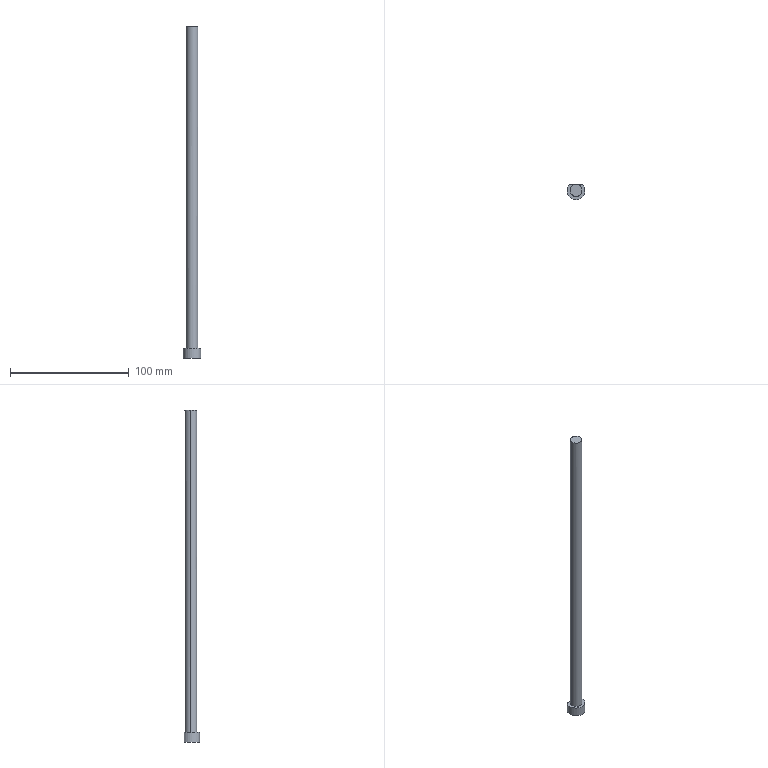Part | Creo | 1 solid | 7 faces | box 15 x 13 x 279.548 mm | volume 22625 mm3 | plane 4 | cylinder 3 | commonest cylinder face diameters 10 x2 15 x1
STEP:
#1=CARTESIAN_POINT('',(0.,0.,0.));
#2=DIRECTION('',(0.,0.,1.));
#3=DIRECTION('',(1.,0.,0.));
#4=AXIS2_PLACEMENT_3D('',#1,#2,#3);
#5=CARTESIAN_POINT('',(39.152,-157.9,-330.441));
#6=VERTEX_POINT('',#5);
#7=CARTESIAN_POINT('',(28.954,-157.9,-330.441));
#8=VERTEX_POINT('',#7);
#9=CARTESIAN_POINT('',(39.152,-157.9,-330.441));
#10=DIRECTION('',(-1.,0.,0.));
#11=VECTOR('',#10,10.198);
#12=LINE('',#9,#11);
#13=EDGE_CURVE('',#6,#8,#12,.T.);
#14=ORIENTED_EDGE('',*,*,#13,.F.);
#15=CARTESIAN_POINT('',(34.053,-163.4,-330.441));
#16=DIRECTION('',(0.,0.,-1.));
#17=DIRECTION('',(0.6799,0.7333,0.));
#18=AXIS2_PLACEMENT_3D('',#15,#16,#17);
#19=CIRCLE('',#18,7.5);
#20=EDGE_CURVE('',#6,#8,#19,.T.);
#21=ORIENTED_EDGE('',*,*,#20,.T.);
#22=EDGE_LOOP('',(#14,#21));
#23=FACE_OUTER_BOUND('',#22,.F.);
#24=CARTESIAN_POINT('',(29.053,-163.4,-330.441));
#25=VERTEX_POINT('',#24);
#26=CARTESIAN_POINT('',(39.053,-163.4,-330.441));
#27=VERTEX_POINT('',#26);
#28=CARTESIAN_POINT('',(34.053,-163.4,-330.441));
#29=DIRECTION('',(0.,0.,-1.));
#30=DIRECTION('',(-1.,0.,0.));
#31=AXIS2_PLACEMENT_3D('',#28,#29,#30);
#32=CIRCLE('',#31,5.);
#33=EDGE_CURVE('',#25,#27,#32,.T.);
#34=ORIENTED_EDGE('',*,*,#33,.F.);
#35=CARTESIAN_POINT('',(34.053,-163.4,-330.441));
#36=DIRECTION('',(0.,0.,-1.));
#37=DIRECTION('',(1.,0.,0.));
#38=AXIS2_PLACEMENT_3D('',#35,#36,#37);
#39=CIRCLE('',#38,5.);
#40=EDGE_CURVE('',#27,#25,#39,.T.);
#41=ORIENTED_EDGE('',*,*,#40,.F.);
#42=EDGE_LOOP('',(#34,#41));
#43=FACE_BOUND('',#42,.F.);
#44=CARTESIAN_POINT('',(34.053,-163.4,-330.441));
#45=DIRECTION('',(0.,0.,-1.));
#46=DIRECTION('',(-1.,0.,0.));
#47=AXIS2_PLACEMENT_3D('',#44,#45,#46);
#48=PLANE('',#47);
#49=ADVANCED_FACE('',(#23,#43),#48,.F.);
#50=CARTESIAN_POINT('',(39.053,-163.4,-58.958));
#51=VERTEX_POINT('',#50);
#52=CARTESIAN_POINT('',(34.383,-158.411,-58.894));
#53=VERTEX_POINT('',#52);
#54=CARTESIAN_POINT('',(39.053,-163.4,-58.958));
#55=CARTESIAN_POINT('',(39.053,-162.62,-58.947));
#56=CARTESIAN_POINT('',(38.729,-161.362,-58.93));
#57=CARTESIAN_POINT('',(37.774,-159.917,-58.911));
#58=CARTESIAN_POINT('',(36.394,-158.868,-58.898));
#59=CARTESIAN_POINT('',(35.161,-158.462,-58.894));
#60=B_SPLINE_CURVE_WITH_KNOTS('',3,(#54,#55,#56,#57,#58,#59,#52),.UNSPECIFIED.,.F.,.F.,(4,1,1,1,4),(0.,0.25,0.5,0.75,1.),.UNSPECIFIED.);
#61=EDGE_CURVE('',#51,#53,#60,.T.);
#62=ORIENTED_EDGE('',*,*,#61,.T.);
#63=CARTESIAN_POINT('',(29.053,-163.4,-58.967));
#64=VERTEX_POINT('',#63);
#65=CARTESIAN_POINT('',(34.383,-158.411,-58.894));
#66=CARTESIAN_POINT('',(33.494,-158.352,-58.894));
#67=CARTESIAN_POINT('',(32.121,-158.665,-58.899));
#68=CARTESIAN_POINT('',(30.559,-159.668,-58.914));
#69=CARTESIAN_POINT('',(29.456,-161.16,-58.936));
#70=CARTESIAN_POINT('',(29.053,-162.509,-58.955));
#71=CARTESIAN_POINT('',(29.053,-163.4,-58.967));
#72=B_SPLINE_CURVE_WITH_KNOTS('',3,(#65,#66,#67,#68,#69,#70,#71),.UNSPECIFIED.,.F.,.F.,(4,1,1,1,4),(0.,0.25,0.5,0.75,1.),.UNSPECIFIED.);
#73=EDGE_CURVE('',#53,#64,#72,.T.);
#74=ORIENTED_EDGE('',*,*,#73,.T.);
#75=CARTESIAN_POINT('',(29.053,-163.4,-330.441));
#76=DIRECTION('',(0.,0.,1.));
#77=VECTOR('',#76,271.475);
#78=LINE('',#75,#77);
#79=EDGE_CURVE('',#25,#64,#78,.T.);
#80=ORIENTED_EDGE('',*,*,#79,.F.);
#81=ORIENTED_EDGE('',*,*,#33,.T.);
#82=CARTESIAN_POINT('',(39.053,-163.4,-330.441));
#83=DIRECTION('',(0.,0.,1.));
#84=VECTOR('',#83,271.484);
#85=LINE('',#82,#84);
#86=EDGE_CURVE('',#27,#51,#85,.T.);
#87=ORIENTED_EDGE('',*,*,#86,.T.);
#88=EDGE_LOOP('',(#62,#74,#80,#81,#87));
#89=FACE_OUTER_BOUND('',#88,.F.);
#90=CARTESIAN_POINT('',(34.053,-163.4,-653.441));
#91=DIRECTION('',(0.,0.,1.));
#92=DIRECTION('',(1.,0.,0.));
#93=AXIS2_PLACEMENT_3D('',#90,#91,#92);
#94=CYLINDRICAL_SURFACE('',#93,5.);
#95=ADVANCED_FACE('',(#89),#94,.T.);
#96=ORIENTED_EDGE('',*,*,#73,.F.);
#97=ORIENTED_EDGE('',*,*,#61,.F.);
#98=CARTESIAN_POINT('',(29.053,-163.4,-58.967));
#99=CARTESIAN_POINT('',(29.053,-163.989,-58.975));
#100=CARTESIAN_POINT('',(29.267,-165.262,-58.992));
#101=CARTESIAN_POINT('',(30.408,-167.041,-59.016));
#102=CARTESIAN_POINT('',(32.203,-168.186,-59.03));
#103=CARTESIAN_POINT('',(34.053,-168.506,-59.032));
#104=CARTESIAN_POINT('',(35.902,-168.186,-59.026));
#105=CARTESIAN_POINT('',(37.697,-167.041,-59.009));
#106=CARTESIAN_POINT('',(38.838,-165.262,-58.984));
#107=CARTESIAN_POINT('',(39.053,-163.989,-58.966));
#108=CARTESIAN_POINT('',(39.053,-163.4,-58.958));
#109=B_SPLINE_CURVE_WITH_KNOTS('',3,(#98,#99,#100,#101,#102,#103,#104,#105,#106,#107,#108),.UNSPECIFIED.,.F.,.F.,(4,1,1,1,1,1,1,1,4),(0.,0.125,0.25,0.375,0.5,0.625,0.75,0.875,1.),.UNSPECIFIED.);
#110=EDGE_CURVE('',#64,#51,#109,.T.);
#111=ORIENTED_EDGE('',*,*,#110,.F.);
#112=EDGE_LOOP('',(#96,#97,#111));
#113=FACE_OUTER_BOUND('',#112,.F.);
#114=CARTESIAN_POINT('',(43.661,-154.909,-58.837));
#115=DIRECTION('',(0.0009063,0.01371,-0.9999));
#116=DIRECTION('',(0.,0.9999,0.01371));
#117=AXIS2_PLACEMENT_3D('',#114,#115,#116);
#118=PLANE('',#117);
#119=ADVANCED_FACE('',(#113),#118,.F.);
#120=ORIENTED_EDGE('',*,*,#110,.T.);
#121=ORIENTED_EDGE('',*,*,#86,.F.);
#122=ORIENTED_EDGE('',*,*,#40,.T.);
#123=ORIENTED_EDGE('',*,*,#79,.T.);
#124=EDGE_LOOP('',(#120,#121,#122,#123));
#125=FACE_OUTER_BOUND('',#124,.F.);
#126=CARTESIAN_POINT('',(34.053,-163.4,-653.441));
#127=DIRECTION('',(0.,0.,1.));
#128=DIRECTION('',(1.,0.,0.));
#129=AXIS2_PLACEMENT_3D('',#126,#127,#128);
#130=CYLINDRICAL_SURFACE('',#129,5.);
#131=ADVANCED_FACE('',(#125),#130,.T.);
#132=CARTESIAN_POINT('',(28.954,-157.9,-338.441));
#133=VERTEX_POINT('',#132);
#134=CARTESIAN_POINT('',(28.954,-157.9,-330.441));
#135=DIRECTION('',(0.,0.,-1.));
#136=VECTOR('',#135,8.);
#137=LINE('',#134,#136);
#138=EDGE_CURVE('',#8,#133,#137,.T.);
#139=ORIENTED_EDGE('',*,*,#138,.T.);
#140=CARTESIAN_POINT('',(39.152,-157.9,-338.441));
#141=VERTEX_POINT('',#140);
#142=CARTESIAN_POINT('',(39.152,-157.9,-338.441));
#143=DIRECTION('',(-1.,0.,0.));
#144=VECTOR('',#143,10.198);
#145=LINE('',#142,#144);
#146=EDGE_CURVE('',#141,#133,#145,.T.);
#147=ORIENTED_EDGE('',*,*,#146,.F.);
#148=CARTESIAN_POINT('',(39.152,-157.9,-338.441));
#149=DIRECTION('',(0.,0.,1.));
#150=VECTOR('',#149,8.);
#151=LINE('',#148,#150);
#152=EDGE_CURVE('',#141,#6,#151,.T.);
#153=ORIENTED_EDGE('',*,*,#152,.T.);
#154=ORIENTED_EDGE('',*,*,#13,.T.);
#155=EDGE_LOOP('',(#139,#147,#153,#154));
#156=FACE_OUTER_BOUND('',#155,.F.);
#157=CARTESIAN_POINT('',(34.053,-157.9,-338.441));
#158=DIRECTION('',(0.,1.,0.));
#159=DIRECTION('',(0.,0.,1.));
#160=AXIS2_PLACEMENT_3D('',#157,#158,#159);
#161=PLANE('',#160);
#162=ADVANCED_FACE('',(#156),#161,.T.);
#163=CARTESIAN_POINT('',(34.053,-163.4,-338.441));
#164=DIRECTION('',(0.,0.,1.));
#165=DIRECTION('',(-0.6799,0.7333,0.));
#166=AXIS2_PLACEMENT_3D('',#163,#164,#165);
#167=CIRCLE('',#166,7.5);
#168=EDGE_CURVE('',#133,#141,#167,.T.);
#169=ORIENTED_EDGE('',*,*,#168,.F.);
#170=ORIENTED_EDGE('',*,*,#138,.F.);
#171=ORIENTED_EDGE('',*,*,#20,.F.);
#172=ORIENTED_EDGE('',*,*,#152,.F.);
#173=EDGE_LOOP('',(#169,#170,#171,#172));
#174=FACE_OUTER_BOUND('',#173,.F.);
#175=CARTESIAN_POINT('',(34.053,-163.4,-330.441));
#176=DIRECTION('',(0.,0.,-1.));
#177=DIRECTION('',(-1.,0.,0.));
#178=AXIS2_PLACEMENT_3D('',#175,#176,#177);
#179=CYLINDRICAL_SURFACE('',#178,7.5);
#180=ADVANCED_FACE('',(#174),#179,.T.);
#181=ORIENTED_EDGE('',*,*,#168,.T.);
#182=ORIENTED_EDGE('',*,*,#146,.T.);
#183=EDGE_LOOP('',(#181,#182));
#184=FACE_OUTER_BOUND('',#183,.F.);
#185=CARTESIAN_POINT('',(71.601,-77.127,-338.441));
#186=DIRECTION('',(0.,0.,-1.));
#187=DIRECTION('',(-1.,0.,0.));
#188=AXIS2_PLACEMENT_3D('',#185,#186,#187);
#189=PLANE('',#188);
#190=ADVANCED_FACE('',(#184),#189,.T.);
#191=CLOSED_SHELL('',(#49,#95,#119,#131,#162,#180,#190));
#192=MANIFOLD_SOLID_BREP('',#191);
#193=(LENGTH_UNIT()NAMED_UNIT(*)SI_UNIT(.MILLI.,.METRE.));
#194=UNCERTAINTY_MEASURE_WITH_UNIT(LENGTH_MEASURE(0.02802),#193,'','');
#195=(NAMED_UNIT(*)PLANE_ANGLE_UNIT()SI_UNIT($,.RADIAN.));
#196=PLANE_ANGLE_MEASURE_WITH_UNIT(PLANE_ANGLE_MEASURE(0.01745),#195);
#197=(CONVERSION_BASED_UNIT('DEGREE',#196)NAMED_UNIT(*)PLANE_ANGLE_UNIT());
#198=(NAMED_UNIT(*)SI_UNIT($,.STERADIAN.)SOLID_ANGLE_UNIT());
#199=(GEOMETRIC_REPRESENTATION_CONTEXT(3)GLOBAL_UNCERTAINTY_ASSIGNED_CONTEXT((#194))GLOBAL_UNIT_ASSIGNED_CONTEXT((#193,#197,#198))REPRESENTATION_CONTEXT('',''));
#200=ADVANCED_BREP_SHAPE_REPRESENTATION('',(#4,#192),#199);